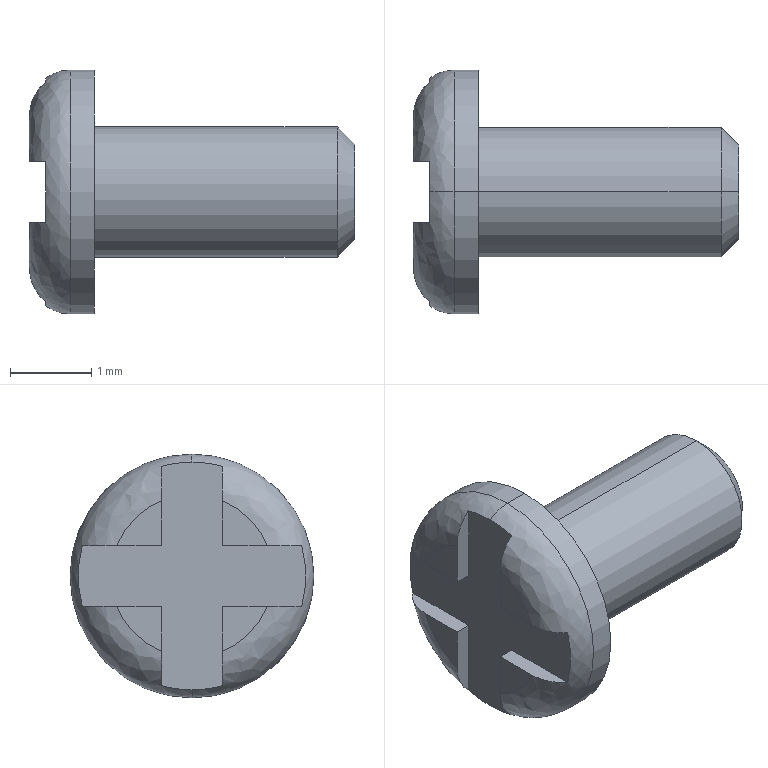Part | STEP file | _Bolt-MG9 | 1 solid | 23 faces | box 4 x 3 x 3 mm | volume 10.872 mm3 | plane 15 | cylinder 4 | spline 2 | cone 2 | commonest cylinder face diameters 1.6 x2 3 x2
STEP:
#1=CARTESIAN_POINT('',(-0.3,0.,1.5));
#2=VERTEX_POINT('',#1);
#3=CARTESIAN_POINT('',(-0.3,0.,-1.5));
#4=VERTEX_POINT('',#3);
#5=CARTESIAN_POINT('',(-0.3,0.,0.));
#6=DIRECTION('',(1.,0.,0.));
#7=DIRECTION('',(0.,0.,1.));
#8=AXIS2_PLACEMENT_3D('',#5,#6,#7);
#9=CIRCLE('',#8,1.5);
#10=EDGE_CURVE('',#2,#4,#9,.T.);
#11=ORIENTED_EDGE('',*,*,#10,.F.);
#12=CARTESIAN_POINT('',(-0.6,0.,1.4));
#13=VERTEX_POINT('',#12);
#14=CARTESIAN_POINT('',(-0.3,0.,1.));
#15=DIRECTION('',(0.,-1.,0.));
#16=DIRECTION('',(0.,0.,1.));
#17=AXIS2_PLACEMENT_3D('',#14,#15,#16);
#18=CIRCLE('',#17,0.5);
#19=EDGE_CURVE('',#2,#13,#18,.T.);
#20=ORIENTED_EDGE('',*,*,#19,.T.);
#21=CARTESIAN_POINT('',(-0.6,-0.375,1.349));
#22=VERTEX_POINT('',#21);
#23=CARTESIAN_POINT('',(-0.6,0.,0.));
#24=DIRECTION('',(1.,0.,0.));
#25=DIRECTION('',(0.,0.,-1.));
#26=AXIS2_PLACEMENT_3D('',#23,#24,#25);
#27=CIRCLE('',#26,1.4);
#28=EDGE_CURVE('',#13,#22,#27,.T.);
#29=ORIENTED_EDGE('',*,*,#28,.T.);
#30=CARTESIAN_POINT('',(-0.8,-0.375,0.927));
#31=VERTEX_POINT('',#30);
#32=CARTESIAN_POINT('',(-0.6,-0.375,1.349));
#33=CARTESIAN_POINT('',(-0.7283,-0.375,1.249));
#34=CARTESIAN_POINT('',(-0.8,-0.375,1.089));
#35=CARTESIAN_POINT('',(-0.8,-0.375,0.927));
#36=B_SPLINE_CURVE_WITH_KNOTS('',3,(#32,#33,#34,#35),.UNSPECIFIED.,.F.,.F.,(4,4),(0.,0.0004804),.UNSPECIFIED.);
#37=EDGE_CURVE('',#22,#31,#36,.T.);
#38=ORIENTED_EDGE('',*,*,#37,.T.);
#39=CARTESIAN_POINT('',(-0.8,-0.927,0.375));
#40=VERTEX_POINT('',#39);
#41=CARTESIAN_POINT('',(-0.8,-0.375,0.927));
#42=CARTESIAN_POINT('',(-0.8,-0.6297,0.824));
#43=CARTESIAN_POINT('',(-0.8,-0.824,0.6297));
#44=CARTESIAN_POINT('',(-0.8,-0.927,0.375));
#45=(BOUNDED_CURVE()B_SPLINE_CURVE(3,(#41,#42,#43,#44),.UNSPECIFIED.,.F.,.T.)B_SPLINE_CURVE_WITH_KNOTS((4,4),(0.,1.),.UNSPECIFIED.)CURVE()GEOMETRIC_REPRESENTATION_ITEM()RATIONAL_B_SPLINE_CURVE((1.,0.9471,0.9471,1.))REPRESENTATION_ITEM(''));
#46=EDGE_CURVE('',#31,#40,#45,.T.);
#47=ORIENTED_EDGE('',*,*,#46,.T.);
#48=CARTESIAN_POINT('',(-0.6,-1.349,0.375));
#49=VERTEX_POINT('',#48);
#50=CARTESIAN_POINT('',(-0.8,-0.927,0.375));
#51=CARTESIAN_POINT('',(-0.8,-1.008,0.375));
#52=CARTESIAN_POINT('',(-0.7828,-1.088,0.375));
#53=CARTESIAN_POINT('',(-0.715,-1.234,0.375));
#54=CARTESIAN_POINT('',(-0.6642,-1.299,0.375));
#55=CARTESIAN_POINT('',(-0.6,-1.349,0.375));
#56=B_SPLINE_CURVE_WITH_KNOTS('',3,(#50,#51,#52,#53,#54,#55),.UNSPECIFIED.,.F.,.F.,(4,2,4),(0.,0.0002403,0.0004806),.UNSPECIFIED.);
#57=EDGE_CURVE('',#40,#49,#56,.T.);
#58=ORIENTED_EDGE('',*,*,#57,.T.);
#59=CARTESIAN_POINT('',(-0.6,-1.349,-0.375));
#60=VERTEX_POINT('',#59);
#61=CARTESIAN_POINT('',(-0.6,0.,0.));
#62=DIRECTION('',(1.,0.,0.));
#63=DIRECTION('',(0.,0.,-1.));
#64=AXIS2_PLACEMENT_3D('',#61,#62,#63);
#65=CIRCLE('',#64,1.4);
#66=EDGE_CURVE('',#49,#60,#65,.T.);
#67=ORIENTED_EDGE('',*,*,#66,.T.);
#68=CARTESIAN_POINT('',(-0.8,-0.927,-0.375));
#69=VERTEX_POINT('',#68);
#70=CARTESIAN_POINT('',(-0.6,-1.349,-0.375));
#71=CARTESIAN_POINT('',(-0.7283,-1.249,-0.375));
#72=CARTESIAN_POINT('',(-0.8,-1.089,-0.375));
#73=CARTESIAN_POINT('',(-0.8,-0.927,-0.375));
#74=B_SPLINE_CURVE_WITH_KNOTS('',3,(#70,#71,#72,#73),.UNSPECIFIED.,.F.,.F.,(4,4),(0.,0.0004804),.UNSPECIFIED.);
#75=EDGE_CURVE('',#60,#69,#74,.T.);
#76=ORIENTED_EDGE('',*,*,#75,.T.);
#77=CARTESIAN_POINT('',(-0.8,-0.375,-0.927));
#78=VERTEX_POINT('',#77);
#79=CARTESIAN_POINT('',(-0.8,-0.927,-0.375));
#80=CARTESIAN_POINT('',(-0.8,-0.824,-0.6297));
#81=CARTESIAN_POINT('',(-0.8,-0.6297,-0.824));
#82=CARTESIAN_POINT('',(-0.8,-0.375,-0.927));
#83=(BOUNDED_CURVE()B_SPLINE_CURVE(3,(#79,#80,#81,#82),.UNSPECIFIED.,.F.,.F.)B_SPLINE_CURVE_WITH_KNOTS((4,4),(0.,1.),.UNSPECIFIED.)CURVE()GEOMETRIC_REPRESENTATION_ITEM()RATIONAL_B_SPLINE_CURVE((1.,0.9471,0.9471,1.))REPRESENTATION_ITEM(''));
#84=EDGE_CURVE('',#69,#78,#83,.T.);
#85=ORIENTED_EDGE('',*,*,#84,.T.);
#86=CARTESIAN_POINT('',(-0.6,-0.375,-1.349));
#87=VERTEX_POINT('',#86);
#88=CARTESIAN_POINT('',(-0.8,-0.375,-0.927));
#89=CARTESIAN_POINT('',(-0.8,-0.375,-1.008));
#90=CARTESIAN_POINT('',(-0.7828,-0.375,-1.088));
#91=CARTESIAN_POINT('',(-0.715,-0.375,-1.234));
#92=CARTESIAN_POINT('',(-0.6642,-0.375,-1.299));
#93=CARTESIAN_POINT('',(-0.6,-0.375,-1.349));
#94=B_SPLINE_CURVE_WITH_KNOTS('',3,(#88,#89,#90,#91,#92,#93),.UNSPECIFIED.,.F.,.F.,(4,2,4),(0.,0.0002403,0.0004806),.UNSPECIFIED.);
#95=EDGE_CURVE('',#78,#87,#94,.T.);
#96=ORIENTED_EDGE('',*,*,#95,.T.);
#97=CARTESIAN_POINT('',(-0.6,0.,-1.4));
#98=VERTEX_POINT('',#97);
#99=CARTESIAN_POINT('',(-0.6,0.,0.));
#100=DIRECTION('',(1.,0.,0.));
#101=DIRECTION('',(0.,0.,-1.));
#102=AXIS2_PLACEMENT_3D('',#99,#100,#101);
#103=CIRCLE('',#102,1.4);
#104=EDGE_CURVE('',#87,#98,#103,.T.);
#105=ORIENTED_EDGE('',*,*,#104,.T.);
#106=CARTESIAN_POINT('',(-0.3,0.,-1.));
#107=DIRECTION('',(0.,1.,0.));
#108=DIRECTION('',(0.,0.,-1.));
#109=AXIS2_PLACEMENT_3D('',#106,#107,#108);
#110=CIRCLE('',#109,0.5);
#111=EDGE_CURVE('',#4,#98,#110,.T.);
#112=ORIENTED_EDGE('',*,*,#111,.F.);
#113=EDGE_LOOP('',(#11,#20,#29,#38,#47,#58,#67,#76,#85,#96,#105,#112));
#114=FACE_OUTER_BOUND('',#113,.T.);
#115=CARTESIAN_POINT('',(-0.3,0.,1.5));
#116=CARTESIAN_POINT('',(-0.3,-3.,1.5));
#117=CARTESIAN_POINT('',(-0.3,-3.,-1.5));
#118=CARTESIAN_POINT('',(-0.3,0.,-1.5));
#119=CARTESIAN_POINT('',(-0.5929,0.,1.5));
#120=CARTESIAN_POINT('',(-0.5929,-3.,1.5));
#121=CARTESIAN_POINT('',(-0.5929,-3.,-1.5));
#122=CARTESIAN_POINT('',(-0.5929,0.,-1.5));
#123=CARTESIAN_POINT('',(-0.8,0.,1.293));
#124=CARTESIAN_POINT('',(-0.8,-2.586,1.293));
#125=CARTESIAN_POINT('',(-0.8,-2.586,-1.293));
#126=CARTESIAN_POINT('',(-0.8,0.,-1.293));
#127=CARTESIAN_POINT('',(-0.8,0.,1.));
#128=CARTESIAN_POINT('',(-0.8,-2.,1.));
#129=CARTESIAN_POINT('',(-0.8,-2.,-1.));
#130=CARTESIAN_POINT('',(-0.8,0.,-1.));
#131=(BOUNDED_SURFACE()B_SPLINE_SURFACE(3,3,((#115,#116,#117,#118),(#119,#120,#121,#122),(#123,#124,#125,#126),(#127,#128,#129,#130)),.UNSPECIFIED.,.F.,.F.,.F.)B_SPLINE_SURFACE_WITH_KNOTS((4,4),(4,4),(0.,1.),(0.,1.),.UNSPECIFIED.)GEOMETRIC_REPRESENTATION_ITEM()RATIONAL_B_SPLINE_SURFACE(((1.,0.3333,0.3333,1.),(0.8047,0.2682,0.2682,0.8047),(0.8047,0.2682,0.2682,0.8047),(1.,0.3333,0.3333,1.)))REPRESENTATION_ITEM('')SURFACE());
#132=ADVANCED_FACE('',(#114),#131,.T.);
#133=CARTESIAN_POINT('',(2.986,0.,0.8));
#134=VERTEX_POINT('',#133);
#135=CARTESIAN_POINT('',(2.986,0.,-0.8));
#136=VERTEX_POINT('',#135);
#137=CARTESIAN_POINT('',(2.986,0.,0.));
#138=DIRECTION('',(-1.,0.,0.));
#139=DIRECTION('',(0.,0.,1.));
#140=AXIS2_PLACEMENT_3D('',#137,#138,#139);
#141=CIRCLE('',#140,0.8);
#142=EDGE_CURVE('',#134,#136,#141,.T.);
#143=ORIENTED_EDGE('',*,*,#142,.T.);
#144=CARTESIAN_POINT('',(0.,0.,-0.8));
#145=VERTEX_POINT('',#144);
#146=CARTESIAN_POINT('',(3.2,0.,-0.8));
#147=DIRECTION('',(-1.,0.,0.));
#148=VECTOR('',#147,1000.);
#149=LINE('',#146,#148);
#150=EDGE_CURVE('',#136,#145,#149,.T.);
#151=ORIENTED_EDGE('',*,*,#150,.T.);
#152=CARTESIAN_POINT('',(0.,0.,0.8));
#153=VERTEX_POINT('',#152);
#154=CARTESIAN_POINT('',(0.,0.,0.));
#155=DIRECTION('',(1.,0.,0.));
#156=DIRECTION('',(0.,0.,1.));
#157=AXIS2_PLACEMENT_3D('',#154,#155,#156);
#158=CIRCLE('',#157,0.8);
#159=EDGE_CURVE('',#145,#153,#158,.T.);
#160=ORIENTED_EDGE('',*,*,#159,.T.);
#161=CARTESIAN_POINT('',(3.2,0.,0.8));
#162=DIRECTION('',(-1.,0.,0.));
#163=VECTOR('',#162,1000.);
#164=LINE('',#161,#163);
#165=EDGE_CURVE('',#134,#153,#164,.T.);
#166=ORIENTED_EDGE('',*,*,#165,.F.);
#167=EDGE_LOOP('',(#143,#151,#160,#166));
#168=FACE_OUTER_BOUND('',#167,.T.);
#169=CARTESIAN_POINT('',(3.2,0.,0.));
#170=DIRECTION('',(-1.,0.,0.));
#171=DIRECTION('',(0.,0.,1.));
#172=AXIS2_PLACEMENT_3D('',#169,#170,#171);
#173=CYLINDRICAL_SURFACE('',#172,0.8);
#174=ADVANCED_FACE('',(#168),#173,.T.);
#175=CARTESIAN_POINT('',(3.2,0.,0.5855));
#176=VERTEX_POINT('',#175);
#177=CARTESIAN_POINT('',(3.2,0.,-0.5855));
#178=VERTEX_POINT('',#177);
#179=CARTESIAN_POINT('',(3.2,0.,0.));
#180=DIRECTION('',(-1.,0.,0.));
#181=DIRECTION('',(0.,0.,1.));
#182=AXIS2_PLACEMENT_3D('',#179,#180,#181);
#183=CIRCLE('',#182,0.5855);
#184=EDGE_CURVE('',#176,#178,#183,.T.);
#185=ORIENTED_EDGE('',*,*,#184,.T.);
#186=CARTESIAN_POINT('',(2.986,0.,-0.8));
#187=DIRECTION('',(-0.7071,0.,-0.7071));
#188=VECTOR('',#187,1000.);
#189=LINE('',#186,#188);
#190=EDGE_CURVE('',#178,#136,#189,.T.);
#191=ORIENTED_EDGE('',*,*,#190,.T.);
#192=ORIENTED_EDGE('',*,*,#142,.F.);
#193=CARTESIAN_POINT('',(2.986,0.,0.8));
#194=DIRECTION('',(-0.7071,0.,0.7071));
#195=VECTOR('',#194,1000.);
#196=LINE('',#193,#195);
#197=EDGE_CURVE('',#176,#134,#196,.T.);
#198=ORIENTED_EDGE('',*,*,#197,.F.);
#199=EDGE_LOOP('',(#185,#191,#192,#198));
#200=FACE_OUTER_BOUND('',#199,.T.);
#201=CARTESIAN_POINT('',(2.986,0.,0.));
#202=DIRECTION('',(-1.,0.,0.));
#203=DIRECTION('',(0.,0.,1.));
#204=AXIS2_PLACEMENT_3D('',#201,#202,#203);
#205=CONICAL_SURFACE('',#204,0.8,0.7854);
#206=ADVANCED_FACE('',(#200),#205,.T.);
#207=CARTESIAN_POINT('',(0.,0.,1.5));
#208=VERTEX_POINT('',#207);
#209=CARTESIAN_POINT('',(0.,0.,-1.5));
#210=VERTEX_POINT('',#209);
#211=CARTESIAN_POINT('',(0.,0.,0.));
#212=DIRECTION('',(-1.,0.,0.));
#213=DIRECTION('',(0.,0.,1.));
#214=AXIS2_PLACEMENT_3D('',#211,#212,#213);
#215=CIRCLE('',#214,1.5);
#216=EDGE_CURVE('',#208,#210,#215,.T.);
#217=ORIENTED_EDGE('',*,*,#216,.T.);
#218=CARTESIAN_POINT('',(3.2,0.,-1.5));
#219=DIRECTION('',(-1.,0.,0.));
#220=VECTOR('',#219,1000.);
#221=LINE('',#218,#220);
#222=EDGE_CURVE('',#210,#4,#221,.T.);
#223=ORIENTED_EDGE('',*,*,#222,.T.);
#224=CARTESIAN_POINT('',(-0.3,0.,0.));
#225=DIRECTION('',(1.,0.,0.));
#226=DIRECTION('',(0.,0.,1.));
#227=AXIS2_PLACEMENT_3D('',#224,#225,#226);
#228=CIRCLE('',#227,1.5);
#229=EDGE_CURVE('',#4,#2,#228,.T.);
#230=ORIENTED_EDGE('',*,*,#229,.T.);
#231=CARTESIAN_POINT('',(3.2,0.,1.5));
#232=DIRECTION('',(-1.,0.,0.));
#233=VECTOR('',#232,1000.);
#234=LINE('',#231,#233);
#235=EDGE_CURVE('',#208,#2,#234,.T.);
#236=ORIENTED_EDGE('',*,*,#235,.F.);
#237=EDGE_LOOP('',(#217,#223,#230,#236));
#238=FACE_OUTER_BOUND('',#237,.T.);
#239=CARTESIAN_POINT('',(3.2,0.,0.));
#240=DIRECTION('',(-1.,0.,0.));
#241=DIRECTION('',(0.,0.,1.));
#242=AXIS2_PLACEMENT_3D('',#239,#240,#241);
#243=CYLINDRICAL_SURFACE('',#242,1.5);
#244=ADVANCED_FACE('',(#238),#243,.T.);
#245=ORIENTED_EDGE('',*,*,#150,.F.);
#246=CARTESIAN_POINT('',(2.986,0.,0.));
#247=DIRECTION('',(-1.,0.,0.));
#248=DIRECTION('',(0.,0.,1.));
#249=AXIS2_PLACEMENT_3D('',#246,#247,#248);
#250=CIRCLE('',#249,0.8);
#251=EDGE_CURVE('',#136,#134,#250,.T.);
#252=ORIENTED_EDGE('',*,*,#251,.T.);
#253=ORIENTED_EDGE('',*,*,#165,.T.);
#254=CARTESIAN_POINT('',(0.,0.,0.));
#255=DIRECTION('',(1.,0.,0.));
#256=DIRECTION('',(0.,0.,1.));
#257=AXIS2_PLACEMENT_3D('',#254,#255,#256);
#258=CIRCLE('',#257,0.8);
#259=EDGE_CURVE('',#153,#145,#258,.T.);
#260=ORIENTED_EDGE('',*,*,#259,.T.);
#261=EDGE_LOOP('',(#245,#252,#253,#260));
#262=FACE_OUTER_BOUND('',#261,.T.);
#263=CARTESIAN_POINT('',(3.2,0.,0.));
#264=DIRECTION('',(-1.,0.,0.));
#265=DIRECTION('',(0.,0.,1.));
#266=AXIS2_PLACEMENT_3D('',#263,#264,#265);
#267=CYLINDRICAL_SURFACE('',#266,0.8);
#268=ADVANCED_FACE('',(#262),#267,.T.);
#269=ORIENTED_EDGE('',*,*,#216,.F.);
#270=CARTESIAN_POINT('',(0.,0.,0.));
#271=DIRECTION('',(-1.,0.,0.));
#272=DIRECTION('',(0.,0.,1.));
#273=AXIS2_PLACEMENT_3D('',#270,#271,#272);
#274=CIRCLE('',#273,1.5);
#275=EDGE_CURVE('',#210,#208,#274,.T.);
#276=ORIENTED_EDGE('',*,*,#275,.F.);
#277=EDGE_LOOP('',(#269,#276));
#278=FACE_OUTER_BOUND('',#277,.T.);
#279=ORIENTED_EDGE('',*,*,#259,.F.);
#280=ORIENTED_EDGE('',*,*,#159,.F.);
#281=EDGE_LOOP('',(#279,#280));
#282=FACE_BOUND('',#281,.T.);
#283=CARTESIAN_POINT('',(0.,1.5,0.));
#284=DIRECTION('',(-1.,0.,0.));
#285=DIRECTION('',(0.,0.,1.));
#286=AXIS2_PLACEMENT_3D('',#283,#284,#285);
#287=PLANE('',#286);
#288=ADVANCED_FACE('',(#278,#282),#287,.F.);
#289=ORIENTED_EDGE('',*,*,#190,.F.);
#290=CARTESIAN_POINT('',(3.2,0.,0.));
#291=DIRECTION('',(-1.,0.,0.));
#292=DIRECTION('',(0.,0.,1.));
#293=AXIS2_PLACEMENT_3D('',#290,#291,#292);
#294=CIRCLE('',#293,0.5855);
#295=EDGE_CURVE('',#178,#176,#294,.T.);
#296=ORIENTED_EDGE('',*,*,#295,.T.);
#297=ORIENTED_EDGE('',*,*,#197,.T.);
#298=ORIENTED_EDGE('',*,*,#251,.F.);
#299=EDGE_LOOP('',(#289,#296,#297,#298));
#300=FACE_OUTER_BOUND('',#299,.T.);
#301=CARTESIAN_POINT('',(2.986,0.,0.));
#302=DIRECTION('',(-1.,0.,0.));
#303=DIRECTION('',(0.,0.,1.));
#304=AXIS2_PLACEMENT_3D('',#301,#302,#303);
#305=CONICAL_SURFACE('',#304,0.8,0.7854);
#306=ADVANCED_FACE('',(#300),#305,.T.);
#307=ORIENTED_EDGE('',*,*,#222,.F.);
#308=ORIENTED_EDGE('',*,*,#275,.T.);
#309=ORIENTED_EDGE('',*,*,#235,.T.);
#310=ORIENTED_EDGE('',*,*,#10,.T.);
#311=EDGE_LOOP('',(#307,#308,#309,#310));
#312=FACE_OUTER_BOUND('',#311,.T.);
#313=CARTESIAN_POINT('',(3.2,0.,0.));
#314=DIRECTION('',(-1.,0.,0.));
#315=DIRECTION('',(0.,0.,1.));
#316=AXIS2_PLACEMENT_3D('',#313,#314,#315);
#317=CYLINDRICAL_SURFACE('',#316,1.5);
#318=ADVANCED_FACE('',(#312),#317,.T.);
#319=ORIENTED_EDGE('',*,*,#184,.F.);
#320=ORIENTED_EDGE('',*,*,#295,.F.);
#321=EDGE_LOOP('',(#319,#320));
#322=FACE_OUTER_BOUND('',#321,.T.);
#323=CARTESIAN_POINT('',(3.2,0.5855,0.));
#324=DIRECTION('',(-1.,0.,0.));
#325=DIRECTION('',(0.,0.,1.));
#326=AXIS2_PLACEMENT_3D('',#323,#324,#325);
#327=PLANE('',#326);
#328=ADVANCED_FACE('',(#322),#327,.F.);
#329=ORIENTED_EDGE('',*,*,#19,.F.);
#330=ORIENTED_EDGE('',*,*,#229,.F.);
#331=ORIENTED_EDGE('',*,*,#111,.T.);
#332=CARTESIAN_POINT('',(-0.6,0.375,-1.349));
#333=VERTEX_POINT('',#332);
#334=CARTESIAN_POINT('',(-0.6,0.,0.));
#335=DIRECTION('',(1.,0.,0.));
#336=DIRECTION('',(0.,0.,-1.));
#337=AXIS2_PLACEMENT_3D('',#334,#335,#336);
#338=CIRCLE('',#337,1.4);
#339=EDGE_CURVE('',#98,#333,#338,.T.);
#340=ORIENTED_EDGE('',*,*,#339,.T.);
#341=CARTESIAN_POINT('',(-0.8,0.375,-0.927));
#342=VERTEX_POINT('',#341);
#343=CARTESIAN_POINT('',(-0.6,0.375,-1.349));
#344=CARTESIAN_POINT('',(-0.7283,0.375,-1.249));
#345=CARTESIAN_POINT('',(-0.8,0.375,-1.089));
#346=CARTESIAN_POINT('',(-0.8,0.375,-0.927));
#347=B_SPLINE_CURVE_WITH_KNOTS('',3,(#343,#344,#345,#346),.UNSPECIFIED.,.F.,.F.,(4,4),(0.,0.0004804),.UNSPECIFIED.);
#348=EDGE_CURVE('',#333,#342,#347,.T.);
#349=ORIENTED_EDGE('',*,*,#348,.T.);
#350=CARTESIAN_POINT('',(-0.8,0.927,-0.375));
#351=VERTEX_POINT('',#350);
#352=CARTESIAN_POINT('',(-0.8,0.375,-0.927));
#353=CARTESIAN_POINT('',(-0.8,0.6297,-0.824));
#354=CARTESIAN_POINT('',(-0.8,0.824,-0.6297));
#355=CARTESIAN_POINT('',(-0.8,0.927,-0.375));
#356=(BOUNDED_CURVE()B_SPLINE_CURVE(3,(#352,#353,#354,#355),.UNSPECIFIED.,.F.,.T.)B_SPLINE_CURVE_WITH_KNOTS((4,4),(0.,1.),.UNSPECIFIED.)CURVE()GEOMETRIC_REPRESENTATION_ITEM()RATIONAL_B_SPLINE_CURVE((1.,0.9471,0.9471,1.))REPRESENTATION_ITEM(''));
#357=EDGE_CURVE('',#342,#351,#356,.T.);
#358=ORIENTED_EDGE('',*,*,#357,.T.);
#359=CARTESIAN_POINT('',(-0.6,1.349,-0.375));
#360=VERTEX_POINT('',#359);
#361=CARTESIAN_POINT('',(-0.8,0.927,-0.375));
#362=CARTESIAN_POINT('',(-0.8,1.008,-0.375));
#363=CARTESIAN_POINT('',(-0.7828,1.088,-0.375));
#364=CARTESIAN_POINT('',(-0.715,1.234,-0.375));
#365=CARTESIAN_POINT('',(-0.6642,1.299,-0.375));
#366=CARTESIAN_POINT('',(-0.6,1.349,-0.375));
#367=B_SPLINE_CURVE_WITH_KNOTS('',3,(#361,#362,#363,#364,#365,#366),.UNSPECIFIED.,.F.,.F.,(4,2,4),(0.,0.0002403,0.0004806),.UNSPECIFIED.);
#368=EDGE_CURVE('',#351,#360,#367,.T.);
#369=ORIENTED_EDGE('',*,*,#368,.T.);
#370=CARTESIAN_POINT('',(-0.6,1.349,0.375));
#371=VERTEX_POINT('',#370);
#372=CARTESIAN_POINT('',(-0.6,0.,0.));
#373=DIRECTION('',(1.,0.,0.));
#374=DIRECTION('',(0.,0.,-1.));
#375=AXIS2_PLACEMENT_3D('',#372,#373,#374);
#376=CIRCLE('',#375,1.4);
#377=EDGE_CURVE('',#360,#371,#376,.T.);
#378=ORIENTED_EDGE('',*,*,#377,.T.);
#379=CARTESIAN_POINT('',(-0.8,0.927,0.375));
#380=VERTEX_POINT('',#379);
#381=CARTESIAN_POINT('',(-0.6,1.349,0.375));
#382=CARTESIAN_POINT('',(-0.7283,1.249,0.375));
#383=CARTESIAN_POINT('',(-0.8,1.089,0.375));
#384=CARTESIAN_POINT('',(-0.8,0.927,0.375));
#385=B_SPLINE_CURVE_WITH_KNOTS('',3,(#381,#382,#383,#384),.UNSPECIFIED.,.F.,.F.,(4,4),(0.,0.0004804),.UNSPECIFIED.);
#386=EDGE_CURVE('',#371,#380,#385,.T.);
#387=ORIENTED_EDGE('',*,*,#386,.T.);
#388=CARTESIAN_POINT('',(-0.8,0.375,0.927));
#389=VERTEX_POINT('',#388);
#390=CARTESIAN_POINT('',(-0.8,0.927,0.375));
#391=CARTESIAN_POINT('',(-0.8,0.824,0.6297));
#392=CARTESIAN_POINT('',(-0.8,0.6297,0.824));
#393=CARTESIAN_POINT('',(-0.8,0.375,0.927));
#394=(BOUNDED_CURVE()B_SPLINE_CURVE(3,(#390,#391,#392,#393),.UNSPECIFIED.,.F.,.F.)B_SPLINE_CURVE_WITH_KNOTS((4,4),(0.,1.),.UNSPECIFIED.)CURVE()GEOMETRIC_REPRESENTATION_ITEM()RATIONAL_B_SPLINE_CURVE((1.,0.9471,0.9471,1.))REPRESENTATION_ITEM(''));
#395=EDGE_CURVE('',#380,#389,#394,.T.);
#396=ORIENTED_EDGE('',*,*,#395,.T.);
#397=CARTESIAN_POINT('',(-0.6,0.375,1.349));
#398=VERTEX_POINT('',#397);
#399=CARTESIAN_POINT('',(-0.8,0.375,0.927));
#400=CARTESIAN_POINT('',(-0.8,0.375,1.008));
#401=CARTESIAN_POINT('',(-0.7828,0.375,1.088));
#402=CARTESIAN_POINT('',(-0.715,0.375,1.234));
#403=CARTESIAN_POINT('',(-0.6642,0.375,1.299));
#404=CARTESIAN_POINT('',(-0.6,0.375,1.349));
#405=B_SPLINE_CURVE_WITH_KNOTS('',3,(#399,#400,#401,#402,#403,#404),.UNSPECIFIED.,.F.,.F.,(4,2,4),(0.,0.0002403,0.0004806),.UNSPECIFIED.);
#406=EDGE_CURVE('',#389,#398,#405,.T.);
#407=ORIENTED_EDGE('',*,*,#406,.T.);
#408=CARTESIAN_POINT('',(-0.6,0.,0.));
#409=DIRECTION('',(1.,0.,0.));
#410=DIRECTION('',(0.,0.,-1.));
#411=AXIS2_PLACEMENT_3D('',#408,#409,#410);
#412=CIRCLE('',#411,1.4);
#413=EDGE_CURVE('',#398,#13,#412,.T.);
#414=ORIENTED_EDGE('',*,*,#413,.T.);
#415=EDGE_LOOP('',(#329,#330,#331,#340,#349,#358,#369,#378,#387,#396,#407,#414));
#416=FACE_OUTER_BOUND('',#415,.T.);
#417=CARTESIAN_POINT('',(-0.3,0.,-1.5));
#418=CARTESIAN_POINT('',(-0.3,3.,-1.5));
#419=CARTESIAN_POINT('',(-0.3,3.,1.5));
#420=CARTESIAN_POINT('',(-0.3,0.,1.5));
#421=CARTESIAN_POINT('',(-0.5929,0.,-1.5));
#422=CARTESIAN_POINT('',(-0.5929,3.,-1.5));
#423=CARTESIAN_POINT('',(-0.5929,3.,1.5));
#424=CARTESIAN_POINT('',(-0.5929,0.,1.5));
#425=CARTESIAN_POINT('',(-0.8,0.,-1.293));
#426=CARTESIAN_POINT('',(-0.8,2.586,-1.293));
#427=CARTESIAN_POINT('',(-0.8,2.586,1.293));
#428=CARTESIAN_POINT('',(-0.8,0.,1.293));
#429=CARTESIAN_POINT('',(-0.8,0.,-1.));
#430=CARTESIAN_POINT('',(-0.8,2.,-1.));
#431=CARTESIAN_POINT('',(-0.8,2.,1.));
#432=CARTESIAN_POINT('',(-0.8,0.,1.));
#433=(BOUNDED_SURFACE()B_SPLINE_SURFACE(3,3,((#417,#418,#419,#420),(#421,#422,#423,#424),(#425,#426,#427,#428),(#429,#430,#431,#432)),.UNSPECIFIED.,.F.,.F.,.F.)B_SPLINE_SURFACE_WITH_KNOTS((4,4),(4,4),(0.,1.),(0.,1.),.UNSPECIFIED.)GEOMETRIC_REPRESENTATION_ITEM()RATIONAL_B_SPLINE_SURFACE(((1.,0.3333,0.3333,1.),(0.8047,0.2682,0.2682,0.8047),(0.8047,0.2682,0.2682,0.8047),(1.,0.3333,0.3333,1.)))REPRESENTATION_ITEM('')SURFACE());
#434=ADVANCED_FACE('',(#416),#433,.T.);
#435=CARTESIAN_POINT('',(-0.6,0.375,-0.375));
#436=VERTEX_POINT('',#435);
#437=CARTESIAN_POINT('',(-0.6,0.375,-0.375));
#438=DIRECTION('',(0.,1.,0.));
#439=VECTOR('',#438,1000.);
#440=LINE('',#437,#439);
#441=EDGE_CURVE('',#436,#360,#440,.T.);
#442=ORIENTED_EDGE('',*,*,#441,.T.);
#443=ORIENTED_EDGE('',*,*,#368,.F.);
#444=CARTESIAN_POINT('',(-0.8,0.375,-0.375));
#445=VERTEX_POINT('',#444);
#446=CARTESIAN_POINT('',(-0.8,0.375,-0.375));
#447=DIRECTION('',(0.,-1.,0.));
#448=VECTOR('',#447,1000.);
#449=LINE('',#446,#448);
#450=EDGE_CURVE('',#351,#445,#449,.T.);
#451=ORIENTED_EDGE('',*,*,#450,.T.);
#452=CARTESIAN_POINT('',(-0.6,0.375,-0.375));
#453=DIRECTION('',(1.,0.,0.));
#454=VECTOR('',#453,1000.);
#455=LINE('',#452,#454);
#456=EDGE_CURVE('',#445,#436,#455,.T.);
#457=ORIENTED_EDGE('',*,*,#456,.T.);
#458=EDGE_LOOP('',(#442,#443,#451,#457));
#459=FACE_OUTER_BOUND('',#458,.T.);
#460=CARTESIAN_POINT('',(-0.6,0.375,-0.375));
#461=DIRECTION('',(0.,0.,1.));
#462=DIRECTION('',(1.,0.,0.));
#463=AXIS2_PLACEMENT_3D('',#460,#461,#462);
#464=PLANE('',#463);
#465=ADVANCED_FACE('',(#459),#464,.T.);
#466=ORIENTED_EDGE('',*,*,#450,.F.);
#467=ORIENTED_EDGE('',*,*,#357,.F.);
#468=CARTESIAN_POINT('',(-0.8,0.375,0.));
#469=DIRECTION('',(0.,0.,-1.));
#470=VECTOR('',#469,1000.);
#471=LINE('',#468,#470);
#472=EDGE_CURVE('',#445,#342,#471,.T.);
#473=ORIENTED_EDGE('',*,*,#472,.F.);
#474=EDGE_LOOP('',(#466,#467,#473));
#475=FACE_OUTER_BOUND('',#474,.T.);
#476=CARTESIAN_POINT('',(-0.8,0.,0.));
#477=DIRECTION('',(1.,0.,0.));
#478=DIRECTION('',(0.,0.,-1.));
#479=AXIS2_PLACEMENT_3D('',#476,#477,#478);
#480=PLANE('',#479);
#481=ADVANCED_FACE('',(#475),#480,.F.);
#482=ORIENTED_EDGE('',*,*,#472,.T.);
#483=ORIENTED_EDGE('',*,*,#348,.F.);
#484=CARTESIAN_POINT('',(-0.6,0.375,-1.452));
#485=DIRECTION('',(0.,0.,1.));
#486=VECTOR('',#485,1000.);
#487=LINE('',#484,#486);
#488=EDGE_CURVE('',#333,#436,#487,.T.);
#489=ORIENTED_EDGE('',*,*,#488,.T.);
#490=ORIENTED_EDGE('',*,*,#456,.F.);
#491=EDGE_LOOP('',(#482,#483,#489,#490));
#492=FACE_OUTER_BOUND('',#491,.T.);
#493=CARTESIAN_POINT('',(-0.6,0.375,-1.452));
#494=DIRECTION('',(0.,-1.,0.));
#495=DIRECTION('',(0.,0.,-1.));
#496=AXIS2_PLACEMENT_3D('',#493,#494,#495);
#497=PLANE('',#496);
#498=ADVANCED_FACE('',(#492),#497,.T.);
#499=CARTESIAN_POINT('',(-0.6,-0.375,0.375));
#500=VERTEX_POINT('',#499);
#501=CARTESIAN_POINT('',(-0.6,0.,0.375));
#502=DIRECTION('',(0.,-1.,0.));
#503=VECTOR('',#502,1000.);
#504=LINE('',#501,#503);
#505=EDGE_CURVE('',#500,#49,#504,.T.);
#506=ORIENTED_EDGE('',*,*,#505,.F.);
#507=CARTESIAN_POINT('',(-0.6,-0.375,0.));
#508=DIRECTION('',(0.,0.,-1.));
#509=VECTOR('',#508,1000.);
#510=LINE('',#507,#509);
#511=EDGE_CURVE('',#22,#500,#510,.T.);
#512=ORIENTED_EDGE('',*,*,#511,.F.);
#513=ORIENTED_EDGE('',*,*,#28,.F.);
#514=ORIENTED_EDGE('',*,*,#413,.F.);
#515=CARTESIAN_POINT('',(-0.6,0.375,0.375));
#516=VERTEX_POINT('',#515);
#517=CARTESIAN_POINT('',(-0.6,0.375,0.));
#518=DIRECTION('',(0.,0.,1.));
#519=VECTOR('',#518,1000.);
#520=LINE('',#517,#519);
#521=EDGE_CURVE('',#516,#398,#520,.T.);
#522=ORIENTED_EDGE('',*,*,#521,.F.);
#523=CARTESIAN_POINT('',(-0.6,0.,0.375));
#524=DIRECTION('',(0.,-1.,0.));
#525=VECTOR('',#524,1000.);
#526=LINE('',#523,#525);
#527=EDGE_CURVE('',#371,#516,#526,.T.);
#528=ORIENTED_EDGE('',*,*,#527,.F.);
#529=ORIENTED_EDGE('',*,*,#377,.F.);
#530=ORIENTED_EDGE('',*,*,#441,.F.);
#531=ORIENTED_EDGE('',*,*,#488,.F.);
#532=ORIENTED_EDGE('',*,*,#339,.F.);
#533=ORIENTED_EDGE('',*,*,#104,.F.);
#534=CARTESIAN_POINT('',(-0.6,-0.375,-0.375));
#535=VERTEX_POINT('',#534);
#536=CARTESIAN_POINT('',(-0.6,-0.375,0.));
#537=DIRECTION('',(0.,0.,-1.));
#538=VECTOR('',#537,1000.);
#539=LINE('',#536,#538);
#540=EDGE_CURVE('',#535,#87,#539,.T.);
#541=ORIENTED_EDGE('',*,*,#540,.F.);
#542=CARTESIAN_POINT('',(-0.6,0.,-0.375));
#543=DIRECTION('',(0.,1.,0.));
#544=VECTOR('',#543,1000.);
#545=LINE('',#542,#544);
#546=EDGE_CURVE('',#60,#535,#545,.T.);
#547=ORIENTED_EDGE('',*,*,#546,.F.);
#548=ORIENTED_EDGE('',*,*,#66,.F.);
#549=EDGE_LOOP('',(#506,#512,#513,#514,#522,#528,#529,#530,#531,#532,#533,#541,#547,#548));
#550=FACE_OUTER_BOUND('',#549,.T.);
#551=CARTESIAN_POINT('',(-0.6,0.,0.));
#552=DIRECTION('',(1.,0.,0.));
#553=DIRECTION('',(0.,0.,-1.));
#554=AXIS2_PLACEMENT_3D('',#551,#552,#553);
#555=PLANE('',#554);
#556=ADVANCED_FACE('',(#550),#555,.F.);
#557=ORIENTED_EDGE('',*,*,#540,.T.);
#558=ORIENTED_EDGE('',*,*,#95,.F.);
#559=CARTESIAN_POINT('',(-0.8,-0.375,-0.375));
#560=VERTEX_POINT('',#559);
#561=CARTESIAN_POINT('',(-0.8,-0.375,-0.375));
#562=DIRECTION('',(0.,0.,1.));
#563=VECTOR('',#562,1000.);
#564=LINE('',#561,#563);
#565=EDGE_CURVE('',#78,#560,#564,.T.);
#566=ORIENTED_EDGE('',*,*,#565,.T.);
#567=CARTESIAN_POINT('',(-0.6,-0.375,-0.375));
#568=DIRECTION('',(1.,0.,0.));
#569=VECTOR('',#568,1000.);
#570=LINE('',#567,#569);
#571=EDGE_CURVE('',#560,#535,#570,.T.);
#572=ORIENTED_EDGE('',*,*,#571,.T.);
#573=EDGE_LOOP('',(#557,#558,#566,#572));
#574=FACE_OUTER_BOUND('',#573,.T.);
#575=CARTESIAN_POINT('',(-0.6,-0.375,-0.375));
#576=DIRECTION('',(0.,1.,0.));
#577=DIRECTION('',(0.,0.,1.));
#578=AXIS2_PLACEMENT_3D('',#575,#576,#577);
#579=PLANE('',#578);
#580=ADVANCED_FACE('',(#574),#579,.T.);
#581=ORIENTED_EDGE('',*,*,#565,.F.);
#582=ORIENTED_EDGE('',*,*,#84,.F.);
#583=CARTESIAN_POINT('',(-0.8,0.,-0.375));
#584=DIRECTION('',(0.,-1.,0.));
#585=VECTOR('',#584,1000.);
#586=LINE('',#583,#585);
#587=EDGE_CURVE('',#560,#69,#586,.T.);
#588=ORIENTED_EDGE('',*,*,#587,.F.);
#589=EDGE_LOOP('',(#581,#582,#588));
#590=FACE_OUTER_BOUND('',#589,.T.);
#591=CARTESIAN_POINT('',(-0.8,0.,0.));
#592=DIRECTION('',(1.,0.,0.));
#593=DIRECTION('',(0.,0.,-1.));
#594=AXIS2_PLACEMENT_3D('',#591,#592,#593);
#595=PLANE('',#594);
#596=ADVANCED_FACE('',(#590),#595,.F.);
#597=ORIENTED_EDGE('',*,*,#587,.T.);
#598=ORIENTED_EDGE('',*,*,#75,.F.);
#599=ORIENTED_EDGE('',*,*,#546,.T.);
#600=ORIENTED_EDGE('',*,*,#571,.F.);
#601=EDGE_LOOP('',(#597,#598,#599,#600));
#602=FACE_OUTER_BOUND('',#601,.T.);
#603=CARTESIAN_POINT('',(-0.6,-1.452,-0.375));
#604=DIRECTION('',(0.,0.,1.));
#605=DIRECTION('',(1.,0.,0.));
#606=AXIS2_PLACEMENT_3D('',#603,#604,#605);
#607=PLANE('',#606);
#608=ADVANCED_FACE('',(#602),#607,.T.);
#609=ORIENTED_EDGE('',*,*,#505,.T.);
#610=ORIENTED_EDGE('',*,*,#57,.F.);
#611=CARTESIAN_POINT('',(-0.8,-0.375,0.375));
#612=VERTEX_POINT('',#611);
#613=CARTESIAN_POINT('',(-0.8,-0.375,0.375));
#614=DIRECTION('',(0.,1.,0.));
#615=VECTOR('',#614,1000.);
#616=LINE('',#613,#615);
#617=EDGE_CURVE('',#40,#612,#616,.T.);
#618=ORIENTED_EDGE('',*,*,#617,.T.);
#619=CARTESIAN_POINT('',(-0.6,-0.375,0.375));
#620=DIRECTION('',(1.,0.,0.));
#621=VECTOR('',#620,1000.);
#622=LINE('',#619,#621);
#623=EDGE_CURVE('',#612,#500,#622,.T.);
#624=ORIENTED_EDGE('',*,*,#623,.T.);
#625=EDGE_LOOP('',(#609,#610,#618,#624));
#626=FACE_OUTER_BOUND('',#625,.T.);
#627=CARTESIAN_POINT('',(-0.6,-0.375,0.375));
#628=DIRECTION('',(0.,0.,-1.));
#629=DIRECTION('',(-1.,0.,0.));
#630=AXIS2_PLACEMENT_3D('',#627,#628,#629);
#631=PLANE('',#630);
#632=ADVANCED_FACE('',(#626),#631,.T.);
#633=ORIENTED_EDGE('',*,*,#617,.F.);
#634=ORIENTED_EDGE('',*,*,#46,.F.);
#635=CARTESIAN_POINT('',(-0.8,-0.375,0.));
#636=DIRECTION('',(0.,0.,1.));
#637=VECTOR('',#636,1000.);
#638=LINE('',#635,#637);
#639=EDGE_CURVE('',#612,#31,#638,.T.);
#640=ORIENTED_EDGE('',*,*,#639,.F.);
#641=EDGE_LOOP('',(#633,#634,#640));
#642=FACE_OUTER_BOUND('',#641,.T.);
#643=CARTESIAN_POINT('',(-0.8,0.,0.));
#644=DIRECTION('',(1.,0.,0.));
#645=DIRECTION('',(0.,0.,-1.));
#646=AXIS2_PLACEMENT_3D('',#643,#644,#645);
#647=PLANE('',#646);
#648=ADVANCED_FACE('',(#642),#647,.F.);
#649=ORIENTED_EDGE('',*,*,#639,.T.);
#650=ORIENTED_EDGE('',*,*,#37,.F.);
#651=ORIENTED_EDGE('',*,*,#511,.T.);
#652=ORIENTED_EDGE('',*,*,#623,.F.);
#653=EDGE_LOOP('',(#649,#650,#651,#652));
#654=FACE_OUTER_BOUND('',#653,.T.);
#655=CARTESIAN_POINT('',(-0.6,-0.375,1.452));
#656=DIRECTION('',(0.,1.,0.));
#657=DIRECTION('',(0.,0.,1.));
#658=AXIS2_PLACEMENT_3D('',#655,#656,#657);
#659=PLANE('',#658);
#660=ADVANCED_FACE('',(#654),#659,.T.);
#661=ORIENTED_EDGE('',*,*,#521,.T.);
#662=ORIENTED_EDGE('',*,*,#406,.F.);
#663=CARTESIAN_POINT('',(-0.8,0.375,0.375));
#664=VERTEX_POINT('',#663);
#665=CARTESIAN_POINT('',(-0.8,0.375,0.375));
#666=DIRECTION('',(0.,0.,-1.));
#667=VECTOR('',#666,1000.);
#668=LINE('',#665,#667);
#669=EDGE_CURVE('',#389,#664,#668,.T.);
#670=ORIENTED_EDGE('',*,*,#669,.T.);
#671=CARTESIAN_POINT('',(-0.6,0.375,0.375));
#672=DIRECTION('',(1.,0.,0.));
#673=VECTOR('',#672,1000.);
#674=LINE('',#671,#673);
#675=EDGE_CURVE('',#664,#516,#674,.T.);
#676=ORIENTED_EDGE('',*,*,#675,.T.);
#677=EDGE_LOOP('',(#661,#662,#670,#676));
#678=FACE_OUTER_BOUND('',#677,.T.);
#679=CARTESIAN_POINT('',(-0.6,0.375,0.375));
#680=DIRECTION('',(0.,-1.,0.));
#681=DIRECTION('',(0.,0.,-1.));
#682=AXIS2_PLACEMENT_3D('',#679,#680,#681);
#683=PLANE('',#682);
#684=ADVANCED_FACE('',(#678),#683,.T.);
#685=ORIENTED_EDGE('',*,*,#395,.F.);
#686=CARTESIAN_POINT('',(-0.8,0.,0.375));
#687=DIRECTION('',(0.,1.,0.));
#688=VECTOR('',#687,1000.);
#689=LINE('',#686,#688);
#690=EDGE_CURVE('',#664,#380,#689,.T.);
#691=ORIENTED_EDGE('',*,*,#690,.F.);
#692=ORIENTED_EDGE('',*,*,#669,.F.);
#693=EDGE_LOOP('',(#685,#691,#692));
#694=FACE_OUTER_BOUND('',#693,.T.);
#695=CARTESIAN_POINT('',(-0.8,0.,0.));
#696=DIRECTION('',(1.,0.,0.));
#697=DIRECTION('',(0.,0.,-1.));
#698=AXIS2_PLACEMENT_3D('',#695,#696,#697);
#699=PLANE('',#698);
#700=ADVANCED_FACE('',(#694),#699,.F.);
#701=ORIENTED_EDGE('',*,*,#690,.T.);
#702=ORIENTED_EDGE('',*,*,#386,.F.);
#703=ORIENTED_EDGE('',*,*,#527,.T.);
#704=ORIENTED_EDGE('',*,*,#675,.F.);
#705=EDGE_LOOP('',(#701,#702,#703,#704));
#706=FACE_OUTER_BOUND('',#705,.T.);
#707=CARTESIAN_POINT('',(-0.6,1.452,0.375));
#708=DIRECTION('',(0.,0.,-1.));
#709=DIRECTION('',(-1.,0.,0.));
#710=AXIS2_PLACEMENT_3D('',#707,#708,#709);
#711=PLANE('',#710);
#712=ADVANCED_FACE('',(#706),#711,.T.);
#713=CLOSED_SHELL('',(#132,#174,#206,#244,#268,#288,#306,#318,#328,#434,#465,#481,#498,#556,#580,#596,#608,#632,#648,#660,#684,#700,#712));
#714=MANIFOLD_SOLID_BREP('',#713);
#715=CARTESIAN_POINT('',(0.,0.,0.));
#716=DIRECTION('',(0.,0.,1.));
#717=DIRECTION('',(1.,0.,0.));
#718=AXIS2_PLACEMENT_3D('',#715,#716,#717);
#719=(LENGTH_UNIT()NAMED_UNIT(*)SI_UNIT(.MILLI.,.METRE.));
#720=UNCERTAINTY_MEASURE_WITH_UNIT(LENGTH_MEASURE(0.00001),#719,'','');
#721=(NAMED_UNIT(*)PLANE_ANGLE_UNIT()SI_UNIT($,.RADIAN.));
#722=(NAMED_UNIT(*)SI_UNIT($,.STERADIAN.)SOLID_ANGLE_UNIT());
#723=(GEOMETRIC_REPRESENTATION_CONTEXT(3)GLOBAL_UNCERTAINTY_ASSIGNED_CONTEXT((#720))GLOBAL_UNIT_ASSIGNED_CONTEXT((#719,#721,#722))REPRESENTATION_CONTEXT('',''));
#724=ADVANCED_BREP_SHAPE_REPRESENTATION('',(#714,#718),#723);